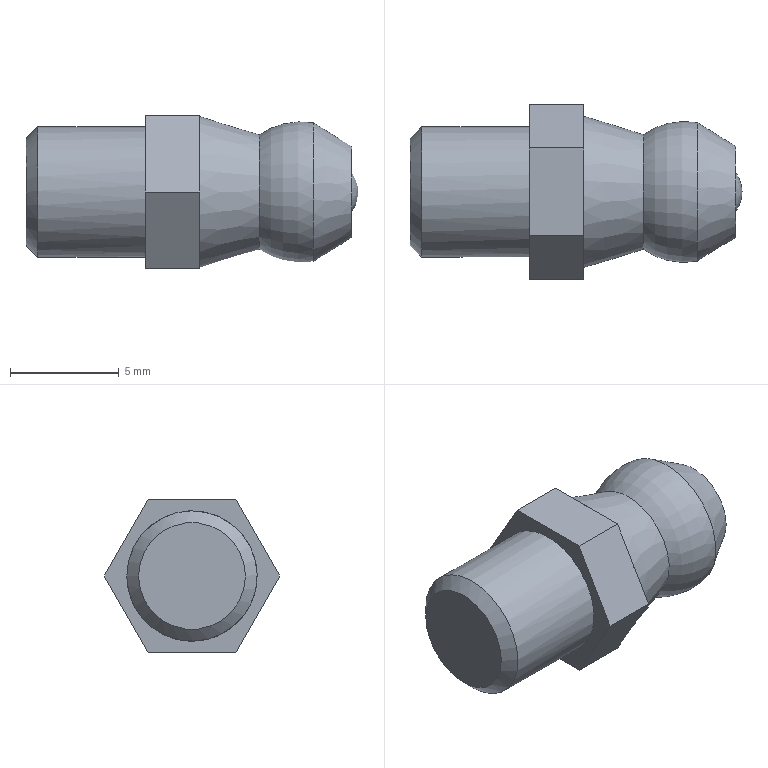Part | STEP file | Grease nipple | 1 solid | 16 faces | box 15.3 x 8.083 x 7 mm | volume 455.493 mm3 | plane 10 | cone 3 | sphere 1 | torus 1 | cylinder 1 | commonest cylinder face diameters 6 x1
STEP:
#1=CARTESIAN_POINT('',(9.5,0.9,0.));
#2=VERTEX_POINT('',#1);
#3=CARTESIAN_POINT('',(9.5,0.,0.));
#4=DIRECTION('',(1.,0.,0.));
#5=DIRECTION('',(0.,1.,0.));
#6=AXIS2_PLACEMENT_3D('',#3,#4,#5);
#7=CIRCLE('',#6,0.9);
#8=EDGE_CURVE('',#2,#2,#7,.T.);
#9=ORIENTED_EDGE('',*,*,#8,.T.);
#10=EDGE_LOOP('',(#9));
#11=FACE_BOUND('',#10,.T.);
#12=CARTESIAN_POINT('',(8.3,0.,0.));
#13=DIRECTION('',(0.,0.,1.));
#14=DIRECTION('',(1.,0.,0.));
#15=AXIS2_PLACEMENT_3D('',#12,#13,#14);
#16=SPHERICAL_SURFACE('',#15,1.5);
#17=ADVANCED_FACE('',(#11),#16,.T.);
#18=CARTESIAN_POINT('',(9.5,2.1,0.));
#19=VERTEX_POINT('',#18);
#20=CARTESIAN_POINT('',(9.5,0.,0.));
#21=DIRECTION('',(1.,0.,0.));
#22=DIRECTION('',(0.,1.,0.));
#23=AXIS2_PLACEMENT_3D('',#20,#21,#22);
#24=CIRCLE('',#23,2.1);
#25=EDGE_CURVE('',#19,#19,#24,.T.);
#26=ORIENTED_EDGE('',*,*,#25,.F.);
#27=EDGE_LOOP('',(#26));
#28=FACE_OUTER_BOUND('',#27,.T.);
#29=CARTESIAN_POINT('',(7.731,3.194,0.));
#30=VERTEX_POINT('',#29);
#31=CARTESIAN_POINT('',(7.731,0.,-3.194));
#32=VERTEX_POINT('',#31);
#33=CARTESIAN_POINT('',(7.731,3.194,0.));
#34=CARTESIAN_POINT('',(7.731,3.194,0.06691));
#35=CARTESIAN_POINT('',(7.731,3.19,0.2007));
#36=CARTESIAN_POINT('',(7.731,3.171,0.4007));
#37=CARTESIAN_POINT('',(7.731,3.14,0.599));
#38=CARTESIAN_POINT('',(7.731,3.096,0.795));
#39=CARTESIAN_POINT('',(7.731,3.04,0.9878));
#40=CARTESIAN_POINT('',(7.731,2.972,1.177));
#41=CARTESIAN_POINT('',(7.731,2.892,1.361));
#42=CARTESIAN_POINT('',(7.731,2.801,1.54));
#43=CARTESIAN_POINT('',(7.731,2.699,1.713));
#44=CARTESIAN_POINT('',(7.731,2.586,1.879));
#45=CARTESIAN_POINT('',(7.731,2.463,2.038));
#46=CARTESIAN_POINT('',(7.731,2.33,2.188));
#47=CARTESIAN_POINT('',(7.731,2.188,2.33));
#48=CARTESIAN_POINT('',(7.731,2.037,2.463));
#49=CARTESIAN_POINT('',(7.731,1.878,2.586));
#50=CARTESIAN_POINT('',(7.731,1.712,2.699));
#51=CARTESIAN_POINT('',(7.731,1.539,2.801));
#52=CARTESIAN_POINT('',(7.731,1.36,2.892));
#53=CARTESIAN_POINT('',(7.731,1.176,2.972));
#54=CARTESIAN_POINT('',(7.731,0.9871,3.04));
#55=CARTESIAN_POINT('',(7.731,0.7942,3.096));
#56=CARTESIAN_POINT('',(7.731,0.5982,3.14));
#57=CARTESIAN_POINT('',(7.731,0.3999,3.171));
#58=CARTESIAN_POINT('',(7.731,0.1999,3.19));
#59=CARTESIAN_POINT('',(7.731,-0.0007991,3.196));
#60=CARTESIAN_POINT('',(7.731,-0.2015,3.19));
#61=CARTESIAN_POINT('',(7.731,-0.4015,3.171));
#62=CARTESIAN_POINT('',(7.731,-0.5998,3.139));
#63=CARTESIAN_POINT('',(7.731,-0.7958,3.096));
#64=CARTESIAN_POINT('',(7.731,-0.9886,3.04));
#65=CARTESIAN_POINT('',(7.731,-1.178,2.971));
#66=CARTESIAN_POINT('',(7.731,-1.362,2.892));
#67=CARTESIAN_POINT('',(7.731,-1.541,2.8));
#68=CARTESIAN_POINT('',(7.731,-1.714,2.698));
#69=CARTESIAN_POINT('',(7.731,-1.88,2.585));
#70=CARTESIAN_POINT('',(7.731,-2.038,2.462));
#71=CARTESIAN_POINT('',(7.731,-2.189,2.329));
#72=CARTESIAN_POINT('',(7.731,-2.331,2.187));
#73=CARTESIAN_POINT('',(7.731,-2.464,2.036));
#74=CARTESIAN_POINT('',(7.731,-2.587,1.878));
#75=CARTESIAN_POINT('',(7.731,-2.699,1.712));
#76=CARTESIAN_POINT('',(7.731,-2.802,1.539));
#77=CARTESIAN_POINT('',(7.731,-2.893,1.36));
#78=CARTESIAN_POINT('',(7.731,-2.972,1.175));
#79=CARTESIAN_POINT('',(7.731,-3.04,0.9863));
#80=CARTESIAN_POINT('',(7.731,-3.096,0.7934));
#81=CARTESIAN_POINT('',(7.731,-3.14,0.5974));
#82=CARTESIAN_POINT('',(7.731,-3.171,0.3991));
#83=CARTESIAN_POINT('',(7.731,-3.19,0.1997));
#84=CARTESIAN_POINT('',(7.731,-3.194,0.06638));
#85=CARTESIAN_POINT('',(7.731,-3.194,0.));
#86=CARTESIAN_POINT('',(7.731,-3.194,-0.06691));
#87=CARTESIAN_POINT('',(7.731,-3.19,-0.2007));
#88=CARTESIAN_POINT('',(7.731,-3.171,-0.4007));
#89=CARTESIAN_POINT('',(7.731,-3.14,-0.599));
#90=CARTESIAN_POINT('',(7.731,-3.096,-0.795));
#91=CARTESIAN_POINT('',(7.731,-3.04,-0.9878));
#92=CARTESIAN_POINT('',(7.731,-2.972,-1.177));
#93=CARTESIAN_POINT('',(7.731,-2.892,-1.361));
#94=CARTESIAN_POINT('',(7.731,-2.801,-1.54));
#95=CARTESIAN_POINT('',(7.731,-2.699,-1.713));
#96=CARTESIAN_POINT('',(7.731,-2.586,-1.879));
#97=CARTESIAN_POINT('',(7.731,-2.463,-2.038));
#98=CARTESIAN_POINT('',(7.731,-2.33,-2.188));
#99=CARTESIAN_POINT('',(7.731,-2.188,-2.33));
#100=CARTESIAN_POINT('',(7.731,-2.037,-2.463));
#101=CARTESIAN_POINT('',(7.731,-1.878,-2.586));
#102=CARTESIAN_POINT('',(7.731,-1.712,-2.699));
#103=CARTESIAN_POINT('',(7.731,-1.539,-2.801));
#104=CARTESIAN_POINT('',(7.731,-1.36,-2.892));
#105=CARTESIAN_POINT('',(7.731,-1.176,-2.972));
#106=CARTESIAN_POINT('',(7.731,-0.9871,-3.04));
#107=CARTESIAN_POINT('',(7.731,-0.7942,-3.096));
#108=CARTESIAN_POINT('',(7.731,-0.5982,-3.14));
#109=CARTESIAN_POINT('',(7.731,-0.3999,-3.171));
#110=CARTESIAN_POINT('',(7.731,-0.2002,-3.19));
#111=CARTESIAN_POINT('',(7.731,-0.06664,-3.194));
#112=CARTESIAN_POINT('',(7.731,0.,-3.194));
#113=B_SPLINE_CURVE_WITH_KNOTS('',3,(#33,#34,#35,#36,#37,#38,#39,#40,#41,#42,#43,#44,#45,#46,#47,#48,#49,#50,#51,#52,#53,#54,#55,#56,#57,#58,#59,#60,#61,#62,#63,#64,#65,#66,#67,#68,#69,#70,#71,#72,#73,#74,#75,#76,#77,#78,#79,#80,#81,#82,#83,#84,#85,#86,#87,#88,#89,#90,#91,#92,#93,#94,#95,#96,#97,#98,#99,#100,#101,#102,#103,#104,#105,#106,#107,#108,#109,#110,#111,#112),.UNSPECIFIED.,.F.,.F.,(4,1,1,1,1,1,1,1,1,1,1,1,1,1,1,1,1,1,1,1,1,1,1,1,1,1,1,1,1,1,1,1,1,1,1,1,1,1,1,1,1,1,1,1,1,1,1,1,1,1,3,1,1,1,1,1,1,1,1,1,1,1,1,1,1,1,1,1,1,1,1,1,1,1,1,4),(0.,0.01334,0.02667,0.04001,0.05334,0.06668,0.08001,0.09335,0.1067,0.12,0.1334,0.1467,0.16,0.1734,0.1867,0.2,0.2134,0.2267,0.24,0.2534,0.2667,0.28,0.2934,0.3067,0.3201,0.3334,0.3467,0.3601,0.3734,0.3867,0.4001,0.4134,0.4267,0.4401,0.4534,0.4667,0.4801,0.4934,0.5067,0.5201,0.5334,0.5468,0.5601,0.5734,0.5868,0.6001,0.6134,0.6268,0.6401,0.6534,0.6667,0.68,0.6933,0.7067,0.72,0.7333,0.7467,0.76,0.7734,0.7867,0.8,0.8134,0.8267,0.84,0.8534,0.8667,0.88,0.8934,0.9067,0.92,0.9334,0.9467,0.96,0.9734,0.9867,1.),.UNSPECIFIED.);
#114=EDGE_CURVE('',#30,#32,#113,.T.);
#115=ORIENTED_EDGE('',*,*,#114,.T.);
#116=CARTESIAN_POINT('',(7.731,0.,0.));
#117=DIRECTION('',(1.,0.,0.));
#118=DIRECTION('',(0.,0.,-1.));
#119=AXIS2_PLACEMENT_3D('',#116,#117,#118);
#120=CIRCLE('',#119,3.194);
#121=EDGE_CURVE('',#32,#30,#120,.T.);
#122=ORIENTED_EDGE('',*,*,#121,.T.);
#123=EDGE_LOOP('',(#115,#122));
#124=FACE_BOUND('',#123,.T.);
#125=CARTESIAN_POINT('',(8.616,0.,0.));
#126=DIRECTION('',(-1.,0.,0.));
#127=DIRECTION('',(0.,1.,0.));
#128=AXIS2_PLACEMENT_3D('',#125,#126,#127);
#129=CONICAL_SURFACE('',#128,2.647,0.554);
#130=ADVANCED_FACE('',(#28,#124),#129,.T.);
#131=ORIENTED_EDGE('',*,*,#121,.F.);
#132=ORIENTED_EDGE('',*,*,#114,.F.);
#133=EDGE_LOOP('',(#131,#132));
#134=FACE_BOUND('',#133,.T.);
#135=CARTESIAN_POINT('',(5.25,2.64,0.));
#136=VERTEX_POINT('',#135);
#137=CARTESIAN_POINT('',(5.25,0.,-2.64));
#138=VERTEX_POINT('',#137);
#139=CARTESIAN_POINT('',(5.25,2.64,0.));
#140=CARTESIAN_POINT('',(5.25,2.64,0.0553));
#141=CARTESIAN_POINT('',(5.25,2.637,0.1659));
#142=CARTESIAN_POINT('',(5.25,2.621,0.3312));
#143=CARTESIAN_POINT('',(5.25,2.595,0.4951));
#144=CARTESIAN_POINT('',(5.25,2.559,0.6571));
#145=CARTESIAN_POINT('',(5.25,2.512,0.8165));
#146=CARTESIAN_POINT('',(5.25,2.456,0.9726));
#147=CARTESIAN_POINT('',(5.25,2.39,1.125));
#148=CARTESIAN_POINT('',(5.25,2.315,1.273));
#149=CARTESIAN_POINT('',(5.25,2.23,1.416));
#150=CARTESIAN_POINT('',(5.25,2.137,1.553));
#151=CARTESIAN_POINT('',(5.25,2.035,1.684));
#152=CARTESIAN_POINT('',(5.25,1.926,1.809));
#153=CARTESIAN_POINT('',(5.25,1.808,1.926));
#154=CARTESIAN_POINT('',(5.25,1.684,2.036));
#155=CARTESIAN_POINT('',(5.25,1.552,2.137));
#156=CARTESIAN_POINT('',(5.25,1.415,2.231));
#157=CARTESIAN_POINT('',(5.25,1.272,2.315));
#158=CARTESIAN_POINT('',(5.25,1.124,2.391));
#159=CARTESIAN_POINT('',(5.25,0.972,2.456));
#160=CARTESIAN_POINT('',(5.25,0.8158,2.513));
#161=CARTESIAN_POINT('',(5.25,0.6564,2.559));
#162=CARTESIAN_POINT('',(5.25,0.4944,2.595));
#163=CARTESIAN_POINT('',(5.25,0.3305,2.621));
#164=CARTESIAN_POINT('',(5.25,0.1652,2.637));
#165=CARTESIAN_POINT('',(5.25,-0.0006604,2.642));
#166=CARTESIAN_POINT('',(5.25,-0.1666,2.636));
#167=CARTESIAN_POINT('',(5.25,-0.3318,2.621));
#168=CARTESIAN_POINT('',(5.25,-0.4957,2.595));
#169=CARTESIAN_POINT('',(5.25,-0.6577,2.559));
#170=CARTESIAN_POINT('',(5.25,-0.8171,2.512));
#171=CARTESIAN_POINT('',(5.25,-0.9733,2.456));
#172=CARTESIAN_POINT('',(5.25,-1.126,2.39));
#173=CARTESIAN_POINT('',(5.25,-1.273,2.315));
#174=CARTESIAN_POINT('',(5.25,-1.416,2.23));
#175=CARTESIAN_POINT('',(5.25,-1.554,2.137));
#176=CARTESIAN_POINT('',(5.25,-1.685,2.035));
#177=CARTESIAN_POINT('',(5.25,-1.809,1.925));
#178=CARTESIAN_POINT('',(5.25,-1.926,1.808));
#179=CARTESIAN_POINT('',(5.25,-2.036,1.683));
#180=CARTESIAN_POINT('',(5.25,-2.138,1.552));
#181=CARTESIAN_POINT('',(5.25,-2.231,1.415));
#182=CARTESIAN_POINT('',(5.25,-2.316,1.272));
#183=CARTESIAN_POINT('',(5.25,-2.391,1.124));
#184=CARTESIAN_POINT('',(5.25,-2.457,0.9714));
#185=CARTESIAN_POINT('',(5.25,-2.513,0.8152));
#186=CARTESIAN_POINT('',(5.25,-2.559,0.6558));
#187=CARTESIAN_POINT('',(5.25,-2.595,0.4938));
#188=CARTESIAN_POINT('',(5.25,-2.621,0.3298));
#189=CARTESIAN_POINT('',(5.25,-2.637,0.165));
#190=CARTESIAN_POINT('',(5.25,-2.64,0.05486));
#191=CARTESIAN_POINT('',(5.25,-2.64,0.));
#192=CARTESIAN_POINT('',(5.25,-2.64,-0.0553));
#193=CARTESIAN_POINT('',(5.25,-2.637,-0.1659));
#194=CARTESIAN_POINT('',(5.25,-2.621,-0.3312));
#195=CARTESIAN_POINT('',(5.25,-2.595,-0.4951));
#196=CARTESIAN_POINT('',(5.25,-2.559,-0.6571));
#197=CARTESIAN_POINT('',(5.25,-2.512,-0.8165));
#198=CARTESIAN_POINT('',(5.25,-2.456,-0.9726));
#199=CARTESIAN_POINT('',(5.25,-2.39,-1.125));
#200=CARTESIAN_POINT('',(5.25,-2.315,-1.273));
#201=CARTESIAN_POINT('',(5.25,-2.23,-1.416));
#202=CARTESIAN_POINT('',(5.25,-2.137,-1.553));
#203=CARTESIAN_POINT('',(5.25,-2.035,-1.684));
#204=CARTESIAN_POINT('',(5.25,-1.926,-1.809));
#205=CARTESIAN_POINT('',(5.25,-1.808,-1.926));
#206=CARTESIAN_POINT('',(5.25,-1.684,-2.036));
#207=CARTESIAN_POINT('',(5.25,-1.552,-2.137));
#208=CARTESIAN_POINT('',(5.25,-1.415,-2.231));
#209=CARTESIAN_POINT('',(5.25,-1.272,-2.315));
#210=CARTESIAN_POINT('',(5.25,-1.124,-2.391));
#211=CARTESIAN_POINT('',(5.25,-0.972,-2.456));
#212=CARTESIAN_POINT('',(5.25,-0.8158,-2.513));
#213=CARTESIAN_POINT('',(5.25,-0.6564,-2.559));
#214=CARTESIAN_POINT('',(5.25,-0.4944,-2.595));
#215=CARTESIAN_POINT('',(5.25,-0.3305,-2.621));
#216=CARTESIAN_POINT('',(5.25,-0.1655,-2.637));
#217=CARTESIAN_POINT('',(5.25,-0.05508,-2.64));
#218=CARTESIAN_POINT('',(5.25,0.,-2.64));
#219=B_SPLINE_CURVE_WITH_KNOTS('',3,(#139,#140,#141,#142,#143,#144,#145,#146,#147,#148,#149,#150,#151,#152,#153,#154,#155,#156,#157,#158,#159,#160,#161,#162,#163,#164,#165,#166,#167,#168,#169,#170,#171,#172,#173,#174,#175,#176,#177,#178,#179,#180,#181,#182,#183,#184,#185,#186,#187,#188,#189,#190,#191,#192,#193,#194,#195,#196,#197,#198,#199,#200,#201,#202,#203,#204,#205,#206,#207,#208,#209,#210,#211,#212,#213,#214,#215,#216,#217,#218),.UNSPECIFIED.,.F.,.F.,(4,1,1,1,1,1,1,1,1,1,1,1,1,1,1,1,1,1,1,1,1,1,1,1,1,1,1,1,1,1,1,1,1,1,1,1,1,1,1,1,1,1,1,1,1,1,1,1,1,1,3,1,1,1,1,1,1,1,1,1,1,1,1,1,1,1,1,1,1,1,1,1,1,1,1,4),(0.,0.01334,0.02667,0.04001,0.05334,0.06668,0.08001,0.09335,0.1067,0.12,0.1334,0.1467,0.16,0.1734,0.1867,0.2,0.2134,0.2267,0.24,0.2534,0.2667,0.28,0.2934,0.3067,0.3201,0.3334,0.3467,0.3601,0.3734,0.3867,0.4001,0.4134,0.4267,0.4401,0.4534,0.4667,0.4801,0.4934,0.5067,0.5201,0.5334,0.5468,0.5601,0.5734,0.5868,0.6001,0.6134,0.6268,0.6401,0.6534,0.6667,0.68,0.6933,0.7067,0.72,0.7333,0.7467,0.76,0.7734,0.7867,0.8,0.8134,0.8267,0.84,0.8534,0.8667,0.88,0.8934,0.9067,0.92,0.9334,0.9467,0.96,0.9734,0.9867,1.),.UNSPECIFIED.);
#220=EDGE_CURVE('',#136,#138,#219,.T.);
#221=ORIENTED_EDGE('',*,*,#220,.T.);
#222=CARTESIAN_POINT('',(5.25,0.,0.));
#223=DIRECTION('',(1.,0.,0.));
#224=DIRECTION('',(0.,0.,-1.));
#225=AXIS2_PLACEMENT_3D('',#222,#223,#224);
#226=CIRCLE('',#225,2.64);
#227=EDGE_CURVE('',#138,#136,#226,.T.);
#228=ORIENTED_EDGE('',*,*,#227,.T.);
#229=EDGE_LOOP('',(#221,#228));
#230=FACE_BOUND('',#229,.T.);
#231=CARTESIAN_POINT('',(7.143,0.,0.));
#232=DIRECTION('',(1.,0.,0.));
#233=DIRECTION('',(0.,0.,-1.));
#234=AXIS2_PLACEMENT_3D('',#231,#232,#233);
#235=DEGENERATE_TOROIDAL_SURFACE('',#234,0.002069,3.25,.F.);
#236=ADVANCED_FACE('',(#134,#230),#235,.F.);
#237=ORIENTED_EDGE('',*,*,#227,.F.);
#238=ORIENTED_EDGE('',*,*,#220,.F.);
#239=EDGE_LOOP('',(#237,#238));
#240=FACE_BOUND('',#239,.T.);
#241=CARTESIAN_POINT('',(2.5,3.49,0.));
#242=VERTEX_POINT('',#241);
#243=CARTESIAN_POINT('',(2.5,0.,0.));
#244=DIRECTION('',(1.,0.,0.));
#245=DIRECTION('',(0.,1.,0.));
#246=AXIS2_PLACEMENT_3D('',#243,#244,#245);
#247=CIRCLE('',#246,3.49);
#248=EDGE_CURVE('',#242,#242,#247,.T.);
#249=ORIENTED_EDGE('',*,*,#248,.T.);
#250=EDGE_LOOP('',(#249));
#251=FACE_OUTER_BOUND('',#250,.T.);
#252=CARTESIAN_POINT('',(3.875,0.,0.));
#253=DIRECTION('',(-1.,0.,0.));
#254=DIRECTION('',(0.,1.,0.));
#255=AXIS2_PLACEMENT_3D('',#252,#253,#254);
#256=CONICAL_SURFACE('',#255,3.065,0.2998);
#257=ADVANCED_FACE('',(#240,#251),#256,.T.);
#258=CARTESIAN_POINT('',(0.,3.,0.));
#259=VERTEX_POINT('',#258);
#260=CARTESIAN_POINT('',(0.,0.,0.));
#261=DIRECTION('',(1.,0.,0.));
#262=DIRECTION('',(0.,1.,0.));
#263=AXIS2_PLACEMENT_3D('',#260,#261,#262);
#264=CIRCLE('',#263,3.);
#265=EDGE_CURVE('',#259,#259,#264,.T.);
#266=ORIENTED_EDGE('',*,*,#265,.F.);
#267=EDGE_LOOP('',(#266));
#268=FACE_OUTER_BOUND('',#267,.T.);
#269=CARTESIAN_POINT('',(-4.959,3.,0.));
#270=VERTEX_POINT('',#269);
#271=CARTESIAN_POINT('',(-4.959,3.,0.));
#272=CARTESIAN_POINT('',(-4.959,3.,0.06284));
#273=CARTESIAN_POINT('',(-4.959,2.996,0.1885));
#274=CARTESIAN_POINT('',(-4.959,2.978,0.3763));
#275=CARTESIAN_POINT('',(-4.959,2.949,0.5626));
#276=CARTESIAN_POINT('',(-4.959,2.908,0.7467));
#277=CARTESIAN_POINT('',(-4.959,2.855,0.9278));
#278=CARTESIAN_POINT('',(-4.959,2.791,1.105));
#279=CARTESIAN_POINT('',(-4.959,2.716,1.278));
#280=CARTESIAN_POINT('',(-4.959,2.631,1.446));
#281=CARTESIAN_POINT('',(-4.959,2.535,1.609));
#282=CARTESIAN_POINT('',(-4.959,2.428,1.765));
#283=CARTESIAN_POINT('',(-4.959,2.313,1.914));
#284=CARTESIAN_POINT('',(-4.959,2.188,2.055));
#285=CARTESIAN_POINT('',(-4.959,2.055,2.189));
#286=CARTESIAN_POINT('',(-4.959,1.913,2.313));
#287=CARTESIAN_POINT('',(-4.959,1.764,2.429));
#288=CARTESIAN_POINT('',(-4.959,1.608,2.535));
#289=CARTESIAN_POINT('',(-4.959,1.446,2.631));
#290=CARTESIAN_POINT('',(-4.959,1.278,2.716));
#291=CARTESIAN_POINT('',(-4.959,1.105,2.791));
#292=CARTESIAN_POINT('',(-4.959,0.9271,2.855));
#293=CARTESIAN_POINT('',(-4.959,0.746,2.908));
#294=CARTESIAN_POINT('',(-4.959,0.5619,2.949));
#295=CARTESIAN_POINT('',(-4.959,0.3756,2.978));
#296=CARTESIAN_POINT('',(-4.959,0.1878,2.996));
#297=CARTESIAN_POINT('',(-4.959,-0.0007505,3.002));
#298=CARTESIAN_POINT('',(-4.959,-0.1893,2.996));
#299=CARTESIAN_POINT('',(-4.959,-0.3771,2.978));
#300=CARTESIAN_POINT('',(-4.959,-0.5633,2.949));
#301=CARTESIAN_POINT('',(-4.959,-0.7474,2.907));
#302=CARTESIAN_POINT('',(-4.959,-0.9285,2.855));
#303=CARTESIAN_POINT('',(-4.959,-1.106,2.791));
#304=CARTESIAN_POINT('',(-4.959,-1.279,2.716));
#305=CARTESIAN_POINT('',(-4.959,-1.447,2.63));
#306=CARTESIAN_POINT('',(-4.959,-1.609,2.534));
#307=CARTESIAN_POINT('',(-4.959,-1.765,2.428));
#308=CARTESIAN_POINT('',(-4.959,-1.914,2.312));
#309=CARTESIAN_POINT('',(-4.959,-2.056,2.188));
#310=CARTESIAN_POINT('',(-4.959,-2.189,2.054));
#311=CARTESIAN_POINT('',(-4.959,-2.314,1.913));
#312=CARTESIAN_POINT('',(-4.959,-2.429,1.764));
#313=CARTESIAN_POINT('',(-4.959,-2.535,1.607));
#314=CARTESIAN_POINT('',(-4.959,-2.631,1.445));
#315=CARTESIAN_POINT('',(-4.959,-2.717,1.277));
#316=CARTESIAN_POINT('',(-4.959,-2.792,1.104));
#317=CARTESIAN_POINT('',(-4.959,-2.855,0.9264));
#318=CARTESIAN_POINT('',(-4.959,-2.908,0.7452));
#319=CARTESIAN_POINT('',(-4.959,-2.949,0.5611));
#320=CARTESIAN_POINT('',(-4.959,-2.978,0.3748));
#321=CARTESIAN_POINT('',(-4.959,-2.996,0.1875));
#322=CARTESIAN_POINT('',(-4.959,-3.,0.06234));
#323=CARTESIAN_POINT('',(-4.959,-3.,0.));
#324=CARTESIAN_POINT('',(-4.959,-3.,-0.06284));
#325=CARTESIAN_POINT('',(-4.959,-2.996,-0.1885));
#326=CARTESIAN_POINT('',(-4.959,-2.978,-0.3763));
#327=CARTESIAN_POINT('',(-4.959,-2.949,-0.5626));
#328=CARTESIAN_POINT('',(-4.959,-2.908,-0.7467));
#329=CARTESIAN_POINT('',(-4.959,-2.855,-0.9278));
#330=CARTESIAN_POINT('',(-4.959,-2.791,-1.105));
#331=CARTESIAN_POINT('',(-4.959,-2.716,-1.278));
#332=CARTESIAN_POINT('',(-4.959,-2.631,-1.446));
#333=CARTESIAN_POINT('',(-4.959,-2.535,-1.609));
#334=CARTESIAN_POINT('',(-4.959,-2.428,-1.765));
#335=CARTESIAN_POINT('',(-4.959,-2.313,-1.914));
#336=CARTESIAN_POINT('',(-4.959,-2.188,-2.055));
#337=CARTESIAN_POINT('',(-4.959,-2.055,-2.189));
#338=CARTESIAN_POINT('',(-4.959,-1.913,-2.313));
#339=CARTESIAN_POINT('',(-4.959,-1.764,-2.429));
#340=CARTESIAN_POINT('',(-4.959,-1.608,-2.535));
#341=CARTESIAN_POINT('',(-4.959,-1.446,-2.631));
#342=CARTESIAN_POINT('',(-4.959,-1.278,-2.716));
#343=CARTESIAN_POINT('',(-4.959,-1.105,-2.791));
#344=CARTESIAN_POINT('',(-4.959,-0.9271,-2.855));
#345=CARTESIAN_POINT('',(-4.959,-0.746,-2.908));
#346=CARTESIAN_POINT('',(-4.959,-0.5619,-2.949));
#347=CARTESIAN_POINT('',(-4.959,-0.3756,-2.978));
#348=CARTESIAN_POINT('',(-4.959,-0.1878,-2.996));
#349=CARTESIAN_POINT('',(-4.959,0.0007505,-3.002));
#350=CARTESIAN_POINT('',(-4.959,0.1893,-2.996));
#351=CARTESIAN_POINT('',(-4.959,0.3771,-2.978));
#352=CARTESIAN_POINT('',(-4.959,0.5633,-2.949));
#353=CARTESIAN_POINT('',(-4.959,0.7474,-2.907));
#354=CARTESIAN_POINT('',(-4.959,0.9285,-2.855));
#355=CARTESIAN_POINT('',(-4.959,1.106,-2.791));
#356=CARTESIAN_POINT('',(-4.959,1.279,-2.716));
#357=CARTESIAN_POINT('',(-4.959,1.447,-2.63));
#358=CARTESIAN_POINT('',(-4.959,1.609,-2.534));
#359=CARTESIAN_POINT('',(-4.959,1.765,-2.428));
#360=CARTESIAN_POINT('',(-4.959,1.914,-2.312));
#361=CARTESIAN_POINT('',(-4.959,2.056,-2.188));
#362=CARTESIAN_POINT('',(-4.959,2.189,-2.054));
#363=CARTESIAN_POINT('',(-4.959,2.314,-1.913));
#364=CARTESIAN_POINT('',(-4.959,2.429,-1.764));
#365=CARTESIAN_POINT('',(-4.959,2.535,-1.607));
#366=CARTESIAN_POINT('',(-4.959,2.631,-1.445));
#367=CARTESIAN_POINT('',(-4.959,2.717,-1.277));
#368=CARTESIAN_POINT('',(-4.959,2.792,-1.104));
#369=CARTESIAN_POINT('',(-4.959,2.855,-0.9264));
#370=CARTESIAN_POINT('',(-4.959,2.908,-0.7452));
#371=CARTESIAN_POINT('',(-4.959,2.949,-0.5611));
#372=CARTESIAN_POINT('',(-4.959,2.978,-0.3748));
#373=CARTESIAN_POINT('',(-4.959,2.996,-0.1875));
#374=CARTESIAN_POINT('',(-4.959,3.,-0.06234));
#375=CARTESIAN_POINT('',(-4.959,3.,0.));
#376=B_SPLINE_CURVE_WITH_KNOTS('',3,(#271,#272,#273,#274,#275,#276,#277,#278,#279,#280,#281,#282,#283,#284,#285,#286,#287,#288,#289,#290,#291,#292,#293,#294,#295,#296,#297,#298,#299,#300,#301,#302,#303,#304,#305,#306,#307,#308,#309,#310,#311,#312,#313,#314,#315,#316,#317,#318,#319,#320,#321,#322,#323,#324,#325,#326,#327,#328,#329,#330,#331,#332,#333,#334,#335,#336,#337,#338,#339,#340,#341,#342,#343,#344,#345,#346,#347,#348,#349,#350,#351,#352,#353,#354,#355,#356,#357,#358,#359,#360,#361,#362,#363,#364,#365,#366,#367,#368,#369,#370,#371,#372,#373,#374,#375),.UNSPECIFIED.,.T.,.F.,(4,1,1,1,1,1,1,1,1,1,1,1,1,1,1,1,1,1,1,1,1,1,1,1,1,1,1,1,1,1,1,1,1,1,1,1,1,1,1,1,1,1,1,1,1,1,1,1,1,1,3,1,1,1,1,1,1,1,1,1,1,1,1,1,1,1,1,1,1,1,1,1,1,1,1,1,1,1,1,1,1,1,1,1,1,1,1,1,1,1,1,1,1,1,1,1,1,1,1,1,4),(0.,0.01,0.02,0.03,0.04001,0.05001,0.06001,0.07001,0.08001,0.09001,0.1,0.11,0.12,0.13,0.14,0.15,0.16,0.17,0.18,0.19,0.2,0.21,0.22,0.23,0.24,0.25,0.26,0.27,0.28,0.29,0.3,0.31,0.3201,0.3301,0.3401,0.3501,0.3601,0.3701,0.3801,0.3901,0.4001,0.4101,0.4201,0.4301,0.4401,0.4501,0.4601,0.4701,0.4801,0.4901,0.5,0.51,0.52,0.53,0.54,0.55,0.56,0.57,0.58,0.59,0.6,0.61,0.62,0.63,0.64,0.65,0.66,0.67,0.68,0.69,0.7,0.71,0.72,0.73,0.74,0.75,0.76,0.77,0.78,0.79,0.8,0.81,0.8201,0.8301,0.8401,0.8501,0.8601,0.8701,0.8801,0.8901,0.9001,0.9101,0.9201,0.9301,0.9401,0.9501,0.9601,0.9701,0.9801,0.9901,1.),.UNSPECIFIED.);
#377=EDGE_CURVE('',#270,#270,#376,.T.);
#378=ORIENTED_EDGE('',*,*,#377,.T.);
#379=EDGE_LOOP('',(#378));
#380=FACE_OUTER_BOUND('',#379,.T.);
#381=CARTESIAN_POINT('',(-2.479,0.,0.));
#382=DIRECTION('',(1.,0.,0.));
#383=DIRECTION('',(0.,1.,0.));
#384=AXIS2_PLACEMENT_3D('',#381,#382,#383);
#385=CYLINDRICAL_SURFACE('',#384,3.);
#386=ADVANCED_FACE('',(#268,#380),#385,.T.);
#387=ORIENTED_EDGE('',*,*,#377,.F.);
#388=EDGE_LOOP('',(#387));
#389=FACE_OUTER_BOUND('',#388,.T.);
#390=CARTESIAN_POINT('',(-5.5,2.459,0.));
#391=VERTEX_POINT('',#390);
#392=CARTESIAN_POINT('',(-5.5,0.,0.));
#393=DIRECTION('',(1.,0.,0.));
#394=DIRECTION('',(0.,-1.,0.));
#395=AXIS2_PLACEMENT_3D('',#392,#393,#394);
#396=CIRCLE('',#395,2.459);
#397=EDGE_CURVE('',#391,#391,#396,.T.);
#398=ORIENTED_EDGE('',*,*,#397,.T.);
#399=EDGE_LOOP('',(#398));
#400=FACE_OUTER_BOUND('',#399,.T.);
#401=CARTESIAN_POINT('',(-5.229,0.,0.));
#402=DIRECTION('',(1.,0.,0.));
#403=DIRECTION('',(0.,1.,0.));
#404=AXIS2_PLACEMENT_3D('',#401,#402,#403);
#405=CONICAL_SURFACE('',#404,2.729,0.7854);
#406=ADVANCED_FACE('',(#389,#400),#405,.T.);
#407=CARTESIAN_POINT('',(0.,4.041,0.));
#408=VERTEX_POINT('',#407);
#409=CARTESIAN_POINT('',(0.,2.021,3.5));
#410=VERTEX_POINT('',#409);
#411=CARTESIAN_POINT('',(0.,4.041,0.));
#412=DIRECTION('',(0.,-0.5,0.866));
#413=VECTOR('',#412,1.);
#414=LINE('',#411,#413);
#415=EDGE_CURVE('',#408,#410,#414,.T.);
#416=ORIENTED_EDGE('',*,*,#415,.T.);
#417=CARTESIAN_POINT('',(2.5,2.021,3.5));
#418=VERTEX_POINT('',#417);
#419=CARTESIAN_POINT('',(0.,2.021,3.5));
#420=DIRECTION('',(1.,0.,0.));
#421=VECTOR('',#420,1.);
#422=LINE('',#419,#421);
#423=EDGE_CURVE('',#410,#418,#422,.T.);
#424=ORIENTED_EDGE('',*,*,#423,.T.);
#425=CARTESIAN_POINT('',(2.5,4.041,0.));
#426=VERTEX_POINT('',#425);
#427=CARTESIAN_POINT('',(2.5,2.021,3.5));
#428=DIRECTION('',(0.,0.5,-0.866));
#429=VECTOR('',#428,1.);
#430=LINE('',#427,#429);
#431=EDGE_CURVE('',#418,#426,#430,.T.);
#432=ORIENTED_EDGE('',*,*,#431,.T.);
#433=CARTESIAN_POINT('',(0.,4.041,0.));
#434=DIRECTION('',(1.,0.,0.));
#435=VECTOR('',#434,1.);
#436=LINE('',#433,#435);
#437=EDGE_CURVE('',#408,#426,#436,.T.);
#438=ORIENTED_EDGE('',*,*,#437,.F.);
#439=EDGE_LOOP('',(#416,#424,#432,#438));
#440=FACE_BOUND('',#439,.T.);
#441=CARTESIAN_POINT('',(0.,3.031,1.75));
#442=DIRECTION('',(0.,0.866,0.5));
#443=DIRECTION('',(0.,-0.5,0.866));
#444=AXIS2_PLACEMENT_3D('',#441,#442,#443);
#445=PLANE('',#444);
#446=ADVANCED_FACE('',(#440),#445,.T.);
#447=CARTESIAN_POINT('',(0.,-2.021,3.5));
#448=VERTEX_POINT('',#447);
#449=CARTESIAN_POINT('',(0.,2.021,3.5));
#450=DIRECTION('',(0.,-1.,0.));
#451=VECTOR('',#450,1.);
#452=LINE('',#449,#451);
#453=EDGE_CURVE('',#410,#448,#452,.T.);
#454=ORIENTED_EDGE('',*,*,#453,.T.);
#455=CARTESIAN_POINT('',(2.5,-2.021,3.5));
#456=VERTEX_POINT('',#455);
#457=CARTESIAN_POINT('',(0.,-2.021,3.5));
#458=DIRECTION('',(1.,0.,0.));
#459=VECTOR('',#458,1.);
#460=LINE('',#457,#459);
#461=EDGE_CURVE('',#448,#456,#460,.T.);
#462=ORIENTED_EDGE('',*,*,#461,.T.);
#463=CARTESIAN_POINT('',(2.5,-2.021,3.5));
#464=DIRECTION('',(0.,1.,0.));
#465=VECTOR('',#464,1.);
#466=LINE('',#463,#465);
#467=EDGE_CURVE('',#456,#418,#466,.T.);
#468=ORIENTED_EDGE('',*,*,#467,.T.);
#469=ORIENTED_EDGE('',*,*,#423,.F.);
#470=EDGE_LOOP('',(#454,#462,#468,#469));
#471=FACE_BOUND('',#470,.T.);
#472=CARTESIAN_POINT('',(0.,0.,3.5));
#473=DIRECTION('',(0.,0.,1.));
#474=DIRECTION('',(0.,-1.,0.));
#475=AXIS2_PLACEMENT_3D('',#472,#473,#474);
#476=PLANE('',#475);
#477=ADVANCED_FACE('',(#471),#476,.T.);
#478=CARTESIAN_POINT('',(0.,-4.041,0.));
#479=VERTEX_POINT('',#478);
#480=CARTESIAN_POINT('',(0.,-2.021,3.5));
#481=DIRECTION('',(0.,-0.5,-0.866));
#482=VECTOR('',#481,1.);
#483=LINE('',#480,#482);
#484=EDGE_CURVE('',#448,#479,#483,.T.);
#485=ORIENTED_EDGE('',*,*,#484,.T.);
#486=CARTESIAN_POINT('',(2.5,-4.041,0.));
#487=VERTEX_POINT('',#486);
#488=CARTESIAN_POINT('',(0.,-4.041,0.));
#489=DIRECTION('',(1.,0.,0.));
#490=VECTOR('',#489,1.);
#491=LINE('',#488,#490);
#492=EDGE_CURVE('',#479,#487,#491,.T.);
#493=ORIENTED_EDGE('',*,*,#492,.T.);
#494=CARTESIAN_POINT('',(2.5,-4.041,0.));
#495=DIRECTION('',(0.,0.5,0.866));
#496=VECTOR('',#495,1.);
#497=LINE('',#494,#496);
#498=EDGE_CURVE('',#487,#456,#497,.T.);
#499=ORIENTED_EDGE('',*,*,#498,.T.);
#500=ORIENTED_EDGE('',*,*,#461,.F.);
#501=EDGE_LOOP('',(#485,#493,#499,#500));
#502=FACE_BOUND('',#501,.T.);
#503=CARTESIAN_POINT('',(0.,-3.031,1.75));
#504=DIRECTION('',(0.,-0.866,0.5));
#505=DIRECTION('',(0.,-0.5,-0.866));
#506=AXIS2_PLACEMENT_3D('',#503,#504,#505);
#507=PLANE('',#506);
#508=ADVANCED_FACE('',(#502),#507,.T.);
#509=CARTESIAN_POINT('',(0.,2.021,-3.5));
#510=VERTEX_POINT('',#509);
#511=CARTESIAN_POINT('',(0.,2.021,-3.5));
#512=DIRECTION('',(0.,0.5,0.866));
#513=VECTOR('',#512,1.);
#514=LINE('',#511,#513);
#515=EDGE_CURVE('',#510,#408,#514,.T.);
#516=ORIENTED_EDGE('',*,*,#515,.T.);
#517=ORIENTED_EDGE('',*,*,#437,.T.);
#518=CARTESIAN_POINT('',(2.5,2.021,-3.5));
#519=VERTEX_POINT('',#518);
#520=CARTESIAN_POINT('',(2.5,4.041,0.));
#521=DIRECTION('',(0.,-0.5,-0.866));
#522=VECTOR('',#521,1.);
#523=LINE('',#520,#522);
#524=EDGE_CURVE('',#426,#519,#523,.T.);
#525=ORIENTED_EDGE('',*,*,#524,.T.);
#526=CARTESIAN_POINT('',(0.,2.021,-3.5));
#527=DIRECTION('',(1.,0.,0.));
#528=VECTOR('',#527,1.);
#529=LINE('',#526,#528);
#530=EDGE_CURVE('',#510,#519,#529,.T.);
#531=ORIENTED_EDGE('',*,*,#530,.F.);
#532=EDGE_LOOP('',(#516,#517,#525,#531));
#533=FACE_BOUND('',#532,.T.);
#534=CARTESIAN_POINT('',(0.,3.031,-1.75));
#535=DIRECTION('',(0.,0.866,-0.5));
#536=DIRECTION('',(0.,0.5,0.866));
#537=AXIS2_PLACEMENT_3D('',#534,#535,#536);
#538=PLANE('',#537);
#539=ADVANCED_FACE('',(#533),#538,.T.);
#540=CARTESIAN_POINT('',(0.,-2.021,-3.5));
#541=VERTEX_POINT('',#540);
#542=CARTESIAN_POINT('',(0.,-2.021,-3.5));
#543=DIRECTION('',(0.,1.,0.));
#544=VECTOR('',#543,1.);
#545=LINE('',#542,#544);
#546=EDGE_CURVE('',#541,#510,#545,.T.);
#547=ORIENTED_EDGE('',*,*,#546,.T.);
#548=ORIENTED_EDGE('',*,*,#530,.T.);
#549=CARTESIAN_POINT('',(2.5,-2.021,-3.5));
#550=VERTEX_POINT('',#549);
#551=CARTESIAN_POINT('',(2.5,2.021,-3.5));
#552=DIRECTION('',(0.,-1.,0.));
#553=VECTOR('',#552,1.);
#554=LINE('',#551,#553);
#555=EDGE_CURVE('',#519,#550,#554,.T.);
#556=ORIENTED_EDGE('',*,*,#555,.T.);
#557=CARTESIAN_POINT('',(0.,-2.021,-3.5));
#558=DIRECTION('',(1.,0.,0.));
#559=VECTOR('',#558,1.);
#560=LINE('',#557,#559);
#561=EDGE_CURVE('',#541,#550,#560,.T.);
#562=ORIENTED_EDGE('',*,*,#561,.F.);
#563=EDGE_LOOP('',(#547,#548,#556,#562));
#564=FACE_BOUND('',#563,.T.);
#565=CARTESIAN_POINT('',(0.,0.,-3.5));
#566=DIRECTION('',(0.,0.,-1.));
#567=DIRECTION('',(0.,1.,0.));
#568=AXIS2_PLACEMENT_3D('',#565,#566,#567);
#569=PLANE('',#568);
#570=ADVANCED_FACE('',(#564),#569,.T.);
#571=CARTESIAN_POINT('',(0.,-4.041,0.));
#572=DIRECTION('',(0.,0.5,-0.866));
#573=VECTOR('',#572,1.);
#574=LINE('',#571,#573);
#575=EDGE_CURVE('',#479,#541,#574,.T.);
#576=ORIENTED_EDGE('',*,*,#575,.T.);
#577=ORIENTED_EDGE('',*,*,#561,.T.);
#578=CARTESIAN_POINT('',(2.5,-2.021,-3.5));
#579=DIRECTION('',(0.,-0.5,0.866));
#580=VECTOR('',#579,1.);
#581=LINE('',#578,#580);
#582=EDGE_CURVE('',#550,#487,#581,.T.);
#583=ORIENTED_EDGE('',*,*,#582,.T.);
#584=ORIENTED_EDGE('',*,*,#492,.F.);
#585=EDGE_LOOP('',(#576,#577,#583,#584));
#586=FACE_BOUND('',#585,.T.);
#587=CARTESIAN_POINT('',(0.,-3.031,-1.75));
#588=DIRECTION('',(0.,-0.866,-0.5));
#589=DIRECTION('',(0.,0.5,-0.866));
#590=AXIS2_PLACEMENT_3D('',#587,#588,#589);
#591=PLANE('',#590);
#592=ADVANCED_FACE('',(#586),#591,.T.);
#593=ORIENTED_EDGE('',*,*,#397,.F.);
#594=EDGE_LOOP('',(#593));
#595=FACE_BOUND('',#594,.T.);
#596=CARTESIAN_POINT('',(-5.5,1.229,0.));
#597=DIRECTION('',(-1.,0.,0.));
#598=DIRECTION('',(0.,-1.,0.));
#599=AXIS2_PLACEMENT_3D('',#596,#597,#598);
#600=PLANE('',#599);
#601=ADVANCED_FACE('',(#595),#600,.T.);
#602=ORIENTED_EDGE('',*,*,#415,.F.);
#603=ORIENTED_EDGE('',*,*,#515,.F.);
#604=ORIENTED_EDGE('',*,*,#546,.F.);
#605=ORIENTED_EDGE('',*,*,#575,.F.);
#606=ORIENTED_EDGE('',*,*,#484,.F.);
#607=ORIENTED_EDGE('',*,*,#453,.F.);
#608=EDGE_LOOP('',(#602,#603,#604,#605,#606,#607));
#609=FACE_BOUND('',#608,.T.);
#610=ORIENTED_EDGE('',*,*,#265,.T.);
#611=EDGE_LOOP('',(#610));
#612=FACE_BOUND('',#611,.T.);
#613=CARTESIAN_POINT('',(0.,3.25,0.));
#614=DIRECTION('',(-1.,0.,0.));
#615=DIRECTION('',(0.,-1.,0.));
#616=AXIS2_PLACEMENT_3D('',#613,#614,#615);
#617=PLANE('',#616);
#618=ADVANCED_FACE('',(#609,#612),#617,.T.);
#619=ORIENTED_EDGE('',*,*,#431,.F.);
#620=ORIENTED_EDGE('',*,*,#467,.F.);
#621=ORIENTED_EDGE('',*,*,#498,.F.);
#622=ORIENTED_EDGE('',*,*,#582,.F.);
#623=ORIENTED_EDGE('',*,*,#555,.F.);
#624=ORIENTED_EDGE('',*,*,#524,.F.);
#625=EDGE_LOOP('',(#619,#620,#621,#622,#623,#624));
#626=FACE_BOUND('',#625,.T.);
#627=ORIENTED_EDGE('',*,*,#248,.F.);
#628=EDGE_LOOP('',(#627));
#629=FACE_BOUND('',#628,.T.);
#630=CARTESIAN_POINT('',(2.5,3.495,0.));
#631=DIRECTION('',(1.,0.,0.));
#632=DIRECTION('',(0.,1.,0.));
#633=AXIS2_PLACEMENT_3D('',#630,#631,#632);
#634=PLANE('',#633);
#635=ADVANCED_FACE('',(#626,#629),#634,.T.);
#636=ORIENTED_EDGE('',*,*,#25,.T.);
#637=EDGE_LOOP('',(#636));
#638=FACE_BOUND('',#637,.T.);
#639=ORIENTED_EDGE('',*,*,#8,.F.);
#640=EDGE_LOOP('',(#639));
#641=FACE_BOUND('',#640,.T.);
#642=CARTESIAN_POINT('',(9.5,1.5,0.));
#643=DIRECTION('',(1.,0.,0.));
#644=DIRECTION('',(0.,1.,0.));
#645=AXIS2_PLACEMENT_3D('',#642,#643,#644);
#646=PLANE('',#645);
#647=ADVANCED_FACE('',(#638,#641),#646,.T.);
#648=CLOSED_SHELL('',(#17,#130,#236,#257,#386,#406,#446,#477,#508,#539,#570,#592,#601,#618,#635,#647));
#649=MANIFOLD_SOLID_BREP('',#648);
#650=(LENGTH_UNIT()NAMED_UNIT(*)SI_UNIT(.MILLI.,.METRE.));
#651=UNCERTAINTY_MEASURE_WITH_UNIT(LENGTH_MEASURE(0.00001),#650,'','');
#652=(NAMED_UNIT(*)PLANE_ANGLE_UNIT()SI_UNIT($,.RADIAN.));
#653=(NAMED_UNIT(*)SI_UNIT($,.STERADIAN.)SOLID_ANGLE_UNIT());
#654=(GEOMETRIC_REPRESENTATION_CONTEXT(3)GLOBAL_UNCERTAINTY_ASSIGNED_CONTEXT((#651))GLOBAL_UNIT_ASSIGNED_CONTEXT((#650,#652,#653))REPRESENTATION_CONTEXT('',''));
#655=ADVANCED_BREP_SHAPE_REPRESENTATION('',(#649),#654);